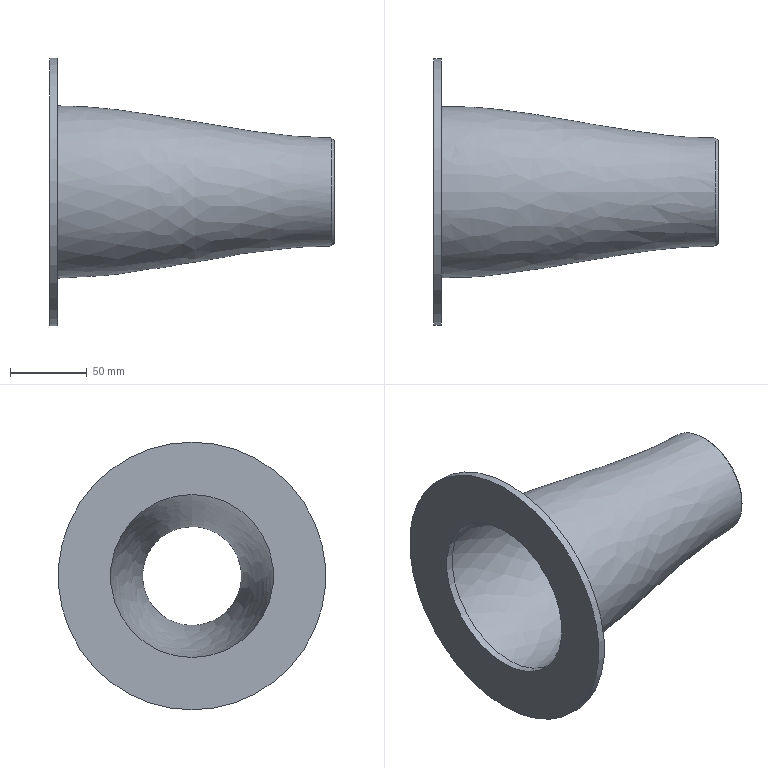Part | STEP file | Reducer Primary Air | 1 solid | 8 faces | box 185 x 174 x 174 mm | volume 225205 mm3 | spline 3 | plane 3 | cylinder 2 | commonest cylinder face diameters 106 x1 174 x1
STEP:
#1=CARTESIAN_POINT('',(-39.149,-5.906,13.134));
#2=VERTEX_POINT('',#1);
#3=CARTESIAN_POINT('',(-39.208,-5.906,13.193));
#4=VERTEX_POINT('',#3);
#5=CARTESIAN_POINT('',(-39.149,-5.906,13.134));
#6=DIRECTION('',(-0.7061,0.,0.7081));
#7=VECTOR('',#6,0.3937);
#8=LINE('',#5,#7);
#9=EDGE_CURVE('',#2,#4,#8,.T.);
#10=ORIENTED_EDGE('',*,*,#9,.T.);
#11=CARTESIAN_POINT('',(-39.208,-5.906,13.193));
#12=CARTESIAN_POINT('',(-39.208,-6.112,13.193));
#13=CARTESIAN_POINT('',(-39.208,-6.526,13.099));
#14=CARTESIAN_POINT('',(-39.208,-7.023,12.702));
#15=CARTESIAN_POINT('',(-39.208,-7.299,12.129));
#16=CARTESIAN_POINT('',(-39.208,-7.299,11.564));
#17=CARTESIAN_POINT('',(-39.208,-7.12,11.11));
#18=CARTESIAN_POINT('',(-39.208,-6.86,10.783));
#19=CARTESIAN_POINT('',(-39.208,-6.572,10.586));
#20=CARTESIAN_POINT('',(-39.208,-6.314,10.485));
#21=CARTESIAN_POINT('',(-39.208,-6.045,10.424));
#22=CARTESIAN_POINT('',(-39.208,-5.696,10.424));
#23=CARTESIAN_POINT('',(-39.208,-5.297,10.547));
#24=CARTESIAN_POINT('',(-39.208,-4.951,10.783));
#25=CARTESIAN_POINT('',(-39.208,-4.69,11.11));
#26=CARTESIAN_POINT('',(-39.208,-4.538,11.499));
#27=CARTESIAN_POINT('',(-39.208,-4.495,12.055));
#28=CARTESIAN_POINT('',(-39.208,-4.732,12.658));
#29=CARTESIAN_POINT('',(-39.208,-5.286,13.099));
#30=CARTESIAN_POINT('',(-39.208,-5.699,13.193));
#31=CARTESIAN_POINT('',(-39.208,-5.906,13.193));
#32=B_SPLINE_CURVE_WITH_KNOTS('',3,(#11,#12,#13,#14,#15,#16,#17,#18,#19,#20,#21,#22,#23,#24,#25,#26,#27,#28,#29,#30,#31),.UNSPECIFIED.,.T.,.F.,(4,1,1,1,1,1,1,1,1,1,1,1,1,1,1,1,1,1,4),(-3.142,-2.693,-2.244,-1.795,-1.346,-1.047,-0.748,-0.4488,-0.2992,-0.1496,0.1496,0.4488,0.748,1.047,1.346,1.646,2.244,2.693,3.142),.UNSPECIFIED.);
#33=EDGE_CURVE('',#4,#4,#32,.T.);
#34=ORIENTED_EDGE('',*,*,#33,.T.);
#35=ORIENTED_EDGE('',*,*,#9,.F.);
#36=CARTESIAN_POINT('',(-39.149,-5.906,13.134));
#37=CARTESIAN_POINT('',(-39.149,-5.708,13.134));
#38=CARTESIAN_POINT('',(-39.149,-5.312,13.043));
#39=CARTESIAN_POINT('',(-39.149,-4.782,12.622));
#40=CARTESIAN_POINT('',(-39.149,-4.556,12.045));
#41=CARTESIAN_POINT('',(-39.149,-4.597,11.512));
#42=CARTESIAN_POINT('',(-39.149,-4.743,11.14));
#43=CARTESIAN_POINT('',(-39.149,-4.992,10.827));
#44=CARTESIAN_POINT('',(-39.149,-5.323,10.601));
#45=CARTESIAN_POINT('',(-39.149,-5.705,10.483));
#46=CARTESIAN_POINT('',(-39.149,-6.039,10.483));
#47=CARTESIAN_POINT('',(-39.149,-6.297,10.542));
#48=CARTESIAN_POINT('',(-39.149,-6.543,10.639));
#49=CARTESIAN_POINT('',(-39.149,-6.819,10.827));
#50=CARTESIAN_POINT('',(-39.149,-7.068,11.14));
#51=CARTESIAN_POINT('',(-39.149,-7.239,11.574));
#52=CARTESIAN_POINT('',(-39.149,-7.239,12.115));
#53=CARTESIAN_POINT('',(-39.149,-6.975,12.664));
#54=CARTESIAN_POINT('',(-39.149,-6.499,13.044));
#55=CARTESIAN_POINT('',(-39.149,-6.103,13.134));
#56=CARTESIAN_POINT('',(-39.149,-5.906,13.134));
#57=B_SPLINE_CURVE_WITH_KNOTS('',3,(#36,#37,#38,#39,#40,#41,#42,#43,#44,#45,#46,#47,#48,#49,#50,#51,#52,#53,#54,#55,#56),.UNSPECIFIED.,.T.,.F.,(4,1,1,1,1,1,1,1,1,1,1,1,1,1,1,1,1,1,4),(-3.142,-2.693,-2.244,-1.646,-1.346,-1.047,-0.748,-0.4488,-0.1496,0.1496,0.2992,0.4488,0.748,1.047,1.346,1.795,2.244,2.693,3.142),.UNSPECIFIED.);
#58=EDGE_CURVE('',#2,#2,#57,.T.);
#59=ORIENTED_EDGE('',*,*,#58,.T.);
#60=EDGE_LOOP('',(#10,#34,#35,#59));
#61=FACE_OUTER_BOUND('',#60,.T.);
#62=CARTESIAN_POINT('',(-39.149,-5.906,13.134));
#63=CARTESIAN_POINT('',(-39.149,-6.103,13.134));
#64=CARTESIAN_POINT('',(-39.149,-6.499,13.044));
#65=CARTESIAN_POINT('',(-39.149,-6.975,12.664));
#66=CARTESIAN_POINT('',(-39.149,-7.239,12.115));
#67=CARTESIAN_POINT('',(-39.149,-7.239,11.574));
#68=CARTESIAN_POINT('',(-39.149,-7.068,11.14));
#69=CARTESIAN_POINT('',(-39.149,-6.819,10.827));
#70=CARTESIAN_POINT('',(-39.149,-6.543,10.639));
#71=CARTESIAN_POINT('',(-39.149,-6.297,10.542));
#72=CARTESIAN_POINT('',(-39.149,-6.039,10.483));
#73=CARTESIAN_POINT('',(-39.149,-5.705,10.483));
#74=CARTESIAN_POINT('',(-39.149,-5.323,10.601));
#75=CARTESIAN_POINT('',(-39.149,-4.992,10.827));
#76=CARTESIAN_POINT('',(-39.149,-4.743,11.14));
#77=CARTESIAN_POINT('',(-39.149,-4.597,11.512));
#78=CARTESIAN_POINT('',(-39.149,-4.556,12.045));
#79=CARTESIAN_POINT('',(-39.149,-4.782,12.622));
#80=CARTESIAN_POINT('',(-39.149,-5.312,13.043));
#81=CARTESIAN_POINT('',(-39.149,-5.708,13.134));
#82=CARTESIAN_POINT('',(-39.149,-5.906,13.134));
#83=CARTESIAN_POINT('',(-39.169,-5.906,13.154));
#84=CARTESIAN_POINT('',(-39.169,-6.106,13.154));
#85=CARTESIAN_POINT('',(-39.169,-6.508,13.062));
#86=CARTESIAN_POINT('',(-39.169,-6.991,12.677));
#87=CARTESIAN_POINT('',(-39.169,-7.259,12.12));
#88=CARTESIAN_POINT('',(-39.169,-7.259,11.571));
#89=CARTESIAN_POINT('',(-39.169,-7.086,11.13));
#90=CARTESIAN_POINT('',(-39.169,-6.832,10.812));
#91=CARTESIAN_POINT('',(-39.169,-6.553,10.621));
#92=CARTESIAN_POINT('',(-39.169,-6.303,10.523));
#93=CARTESIAN_POINT('',(-39.169,-6.041,10.463));
#94=CARTESIAN_POINT('',(-39.169,-5.702,10.463));
#95=CARTESIAN_POINT('',(-39.169,-5.314,10.583));
#96=CARTESIAN_POINT('',(-39.169,-4.979,10.812));
#97=CARTESIAN_POINT('',(-39.169,-4.725,11.13));
#98=CARTESIAN_POINT('',(-39.169,-4.577,11.508));
#99=CARTESIAN_POINT('',(-39.169,-4.536,12.048));
#100=CARTESIAN_POINT('',(-39.169,-4.765,12.634));
#101=CARTESIAN_POINT('',(-39.169,-5.304,13.062));
#102=CARTESIAN_POINT('',(-39.169,-5.705,13.154));
#103=CARTESIAN_POINT('',(-39.169,-5.906,13.154));
#104=CARTESIAN_POINT('',(-39.189,-5.906,13.173));
#105=CARTESIAN_POINT('',(-39.189,-6.109,13.173));
#106=CARTESIAN_POINT('',(-39.189,-6.517,13.08));
#107=CARTESIAN_POINT('',(-39.189,-7.007,12.689));
#108=CARTESIAN_POINT('',(-39.189,-7.279,12.124));
#109=CARTESIAN_POINT('',(-39.189,-7.279,11.567));
#110=CARTESIAN_POINT('',(-39.189,-7.103,11.12));
#111=CARTESIAN_POINT('',(-39.189,-6.846,10.797));
#112=CARTESIAN_POINT('',(-39.189,-6.562,10.604));
#113=CARTESIAN_POINT('',(-39.189,-6.309,10.504));
#114=CARTESIAN_POINT('',(-39.189,-6.043,10.444));
#115=CARTESIAN_POINT('',(-39.189,-5.699,10.444));
#116=CARTESIAN_POINT('',(-39.189,-5.305,10.565));
#117=CARTESIAN_POINT('',(-39.189,-4.965,10.797));
#118=CARTESIAN_POINT('',(-39.189,-4.708,11.12));
#119=CARTESIAN_POINT('',(-39.189,-4.558,11.503));
#120=CARTESIAN_POINT('',(-39.189,-4.515,12.052));
#121=CARTESIAN_POINT('',(-39.189,-4.749,12.646));
#122=CARTESIAN_POINT('',(-39.189,-5.295,13.08));
#123=CARTESIAN_POINT('',(-39.189,-5.702,13.173));
#124=CARTESIAN_POINT('',(-39.189,-5.906,13.173));
#125=CARTESIAN_POINT('',(-39.208,-5.906,13.193));
#126=CARTESIAN_POINT('',(-39.208,-6.112,13.193));
#127=CARTESIAN_POINT('',(-39.208,-6.526,13.099));
#128=CARTESIAN_POINT('',(-39.208,-7.023,12.702));
#129=CARTESIAN_POINT('',(-39.208,-7.299,12.129));
#130=CARTESIAN_POINT('',(-39.208,-7.299,11.564));
#131=CARTESIAN_POINT('',(-39.208,-7.12,11.11));
#132=CARTESIAN_POINT('',(-39.208,-6.86,10.783));
#133=CARTESIAN_POINT('',(-39.208,-6.572,10.586));
#134=CARTESIAN_POINT('',(-39.208,-6.314,10.485));
#135=CARTESIAN_POINT('',(-39.208,-6.045,10.424));
#136=CARTESIAN_POINT('',(-39.208,-5.696,10.424));
#137=CARTESIAN_POINT('',(-39.208,-5.297,10.547));
#138=CARTESIAN_POINT('',(-39.208,-4.951,10.783));
#139=CARTESIAN_POINT('',(-39.208,-4.69,11.11));
#140=CARTESIAN_POINT('',(-39.208,-4.538,11.499));
#141=CARTESIAN_POINT('',(-39.208,-4.495,12.055));
#142=CARTESIAN_POINT('',(-39.208,-4.732,12.658));
#143=CARTESIAN_POINT('',(-39.208,-5.286,13.099));
#144=CARTESIAN_POINT('',(-39.208,-5.699,13.193));
#145=CARTESIAN_POINT('',(-39.208,-5.906,13.193));
#146=B_SPLINE_SURFACE_WITH_KNOTS('',3,3,((#62,#63,#64,#65,#66,#67,#68,#69,#70,#71,#72,#73,#74,#75,#76,#77,#78,#79,#80,#81,#82),(#83,#84,#85,#86,#87,#88,#89,#90,#91,#92,#93,#94,#95,#96,#97,#98,#99,#100,#101,#102,#103),(#104,#105,#106,#107,#108,#109,#110,#111,#112,#113,#114,#115,#116,#117,#118,#119,#120,#121,#122,#123,#124),(#125,#126,#127,#128,#129,#130,#131,#132,#133,#134,#135,#136,#137,#138,#139,#140,#141,#142,#143,#144,#145)),.UNSPECIFIED.,.F.,.T.,.F.,(4,4),(4,1,1,1,1,1,1,1,1,1,1,1,1,1,1,1,1,1,4),(0.,1.),(-3.142,-2.693,-2.244,-1.795,-1.346,-1.047,-0.748,-0.4488,-0.2992,-0.1496,0.1496,0.4488,0.748,1.047,1.346,1.646,2.244,2.693,3.142),.UNSPECIFIED.);
#147=ADVANCED_FACE('',(#61),#146,.T.);
#148=ORIENTED_EDGE('',*,*,#33,.F.);
#149=CARTESIAN_POINT('',(-46.236,-5.906,14.016));
#150=VERTEX_POINT('',#149);
#151=CARTESIAN_POINT('',(-39.208,-5.906,13.193));
#152=CARTESIAN_POINT('',(-41.551,-5.906,13.207));
#153=CARTESIAN_POINT('',(-43.893,-5.906,14.016));
#154=CARTESIAN_POINT('',(-46.236,-5.906,14.016));
#155=B_SPLINE_CURVE_WITH_KNOTS('',3,(#151,#152,#153,#154),.UNSPECIFIED.,.F.,.F.,(4,4),(0.008333,1.),.UNSPECIFIED.);
#156=EDGE_CURVE('',#4,#150,#155,.T.);
#157=ORIENTED_EDGE('',*,*,#156,.T.);
#158=CARTESIAN_POINT('',(-46.236,-5.906,11.811));
#159=DIRECTION('',(1.,0.,0.));
#160=DIRECTION('',(0.,0.,-1.));
#161=AXIS2_PLACEMENT_3D('',#158,#159,#160);
#162=CIRCLE('',#161,2.205);
#163=EDGE_CURVE('',#150,#150,#162,.T.);
#164=ORIENTED_EDGE('',*,*,#163,.T.);
#165=ORIENTED_EDGE('',*,*,#156,.F.);
#166=EDGE_LOOP('',(#148,#157,#164,#165));
#167=FACE_OUTER_BOUND('',#166,.T.);
#168=CARTESIAN_POINT('',(-39.208,-5.906,13.193));
#169=CARTESIAN_POINT('',(-41.551,-5.906,13.207));
#170=CARTESIAN_POINT('',(-43.893,-5.906,14.016));
#171=CARTESIAN_POINT('',(-46.236,-5.906,14.016));
#172=CARTESIAN_POINT('',(-39.208,-6.112,13.193));
#173=CARTESIAN_POINT('',(-41.551,-6.114,13.207));
#174=CARTESIAN_POINT('',(-43.893,-6.235,14.016));
#175=CARTESIAN_POINT('',(-46.236,-6.235,14.016));
#176=CARTESIAN_POINT('',(-39.208,-6.526,13.099));
#177=CARTESIAN_POINT('',(-41.551,-6.532,13.111));
#178=CARTESIAN_POINT('',(-43.893,-6.895,13.865));
#179=CARTESIAN_POINT('',(-46.236,-6.895,13.865));
#180=CARTESIAN_POINT('',(-39.208,-6.968,12.746));
#181=CARTESIAN_POINT('',(-41.551,-6.978,12.755));
#182=CARTESIAN_POINT('',(-43.893,-7.6,13.303));
#183=CARTESIAN_POINT('',(-46.236,-7.6,13.303));
#184=CARTESIAN_POINT('',(-39.208,-7.211,12.323));
#185=CARTESIAN_POINT('',(-41.551,-7.224,12.328));
#186=CARTESIAN_POINT('',(-43.893,-7.989,12.628));
#187=CARTESIAN_POINT('',(-46.236,-7.989,12.628));
#188=CARTESIAN_POINT('',(-39.208,-7.304,11.916));
#189=CARTESIAN_POINT('',(-41.551,-7.318,11.917));
#190=CARTESIAN_POINT('',(-43.893,-8.137,11.978));
#191=CARTESIAN_POINT('',(-46.236,-8.137,11.978));
#192=CARTESIAN_POINT('',(-39.208,-7.273,11.499));
#193=CARTESIAN_POINT('',(-41.551,-7.286,11.496));
#194=CARTESIAN_POINT('',(-43.893,-8.087,11.313));
#195=CARTESIAN_POINT('',(-46.236,-8.087,11.313));
#196=CARTESIAN_POINT('',(-39.208,-7.12,11.11));
#197=CARTESIAN_POINT('',(-41.551,-7.132,11.103));
#198=CARTESIAN_POINT('',(-43.893,-7.844,10.692));
#199=CARTESIAN_POINT('',(-46.236,-7.844,10.692));
#200=CARTESIAN_POINT('',(-39.208,-6.86,10.783));
#201=CARTESIAN_POINT('',(-41.551,-6.869,10.773));
#202=CARTESIAN_POINT('',(-43.893,-7.428,10.171));
#203=CARTESIAN_POINT('',(-46.236,-7.428,10.171));
#204=CARTESIAN_POINT('',(-39.208,-6.514,10.547));
#205=CARTESIAN_POINT('',(-41.551,-6.52,10.535));
#206=CARTESIAN_POINT('',(-43.893,-6.876,9.795));
#207=CARTESIAN_POINT('',(-46.236,-6.876,9.795));
#208=CARTESIAN_POINT('',(-39.208,-6.115,10.424));
#209=CARTESIAN_POINT('',(-41.551,-6.117,10.41));
#210=CARTESIAN_POINT('',(-43.893,-6.239,9.598));
#211=CARTESIAN_POINT('',(-46.236,-6.239,9.598));
#212=CARTESIAN_POINT('',(-39.208,-5.696,10.424));
#213=CARTESIAN_POINT('',(-41.551,-5.694,10.41));
#214=CARTESIAN_POINT('',(-43.893,-5.572,9.598));
#215=CARTESIAN_POINT('',(-46.236,-5.572,9.598));
#216=CARTESIAN_POINT('',(-39.208,-5.297,10.547));
#217=CARTESIAN_POINT('',(-41.551,-5.291,10.535));
#218=CARTESIAN_POINT('',(-43.893,-4.934,9.795));
#219=CARTESIAN_POINT('',(-46.236,-4.934,9.795));
#220=CARTESIAN_POINT('',(-39.208,-4.951,10.783));
#221=CARTESIAN_POINT('',(-41.551,-4.942,10.773));
#222=CARTESIAN_POINT('',(-43.893,-4.383,10.17));
#223=CARTESIAN_POINT('',(-46.236,-4.383,10.17));
#224=CARTESIAN_POINT('',(-39.208,-4.691,11.11));
#225=CARTESIAN_POINT('',(-41.551,-4.679,11.103));
#226=CARTESIAN_POINT('',(-43.893,-3.967,10.692));
#227=CARTESIAN_POINT('',(-46.236,-3.967,10.692));
#228=CARTESIAN_POINT('',(-39.208,-4.512,11.564));
#229=CARTESIAN_POINT('',(-41.551,-4.499,11.561));
#230=CARTESIAN_POINT('',(-43.893,-3.683,11.416));
#231=CARTESIAN_POINT('',(-46.236,-3.683,11.416));
#232=CARTESIAN_POINT('',(-39.208,-4.512,12.129));
#233=CARTESIAN_POINT('',(-41.551,-4.498,12.132));
#234=CARTESIAN_POINT('',(-43.893,-3.683,12.318));
#235=CARTESIAN_POINT('',(-46.236,-3.683,12.318));
#236=CARTESIAN_POINT('',(-39.208,-4.788,12.702));
#237=CARTESIAN_POINT('',(-41.551,-4.777,12.711));
#238=CARTESIAN_POINT('',(-43.893,-4.123,13.233));
#239=CARTESIAN_POINT('',(-46.236,-4.123,13.233));
#240=CARTESIAN_POINT('',(-39.208,-5.285,13.099));
#241=CARTESIAN_POINT('',(-41.551,-5.279,13.111));
#242=CARTESIAN_POINT('',(-43.893,-4.916,13.865));
#243=CARTESIAN_POINT('',(-46.236,-4.916,13.865));
#244=CARTESIAN_POINT('',(-39.208,-5.699,13.193));
#245=CARTESIAN_POINT('',(-41.551,-5.697,13.207));
#246=CARTESIAN_POINT('',(-43.893,-5.576,14.016));
#247=CARTESIAN_POINT('',(-46.236,-5.576,14.016));
#248=CARTESIAN_POINT('',(-39.208,-5.906,13.193));
#249=CARTESIAN_POINT('',(-41.551,-5.906,13.207));
#250=CARTESIAN_POINT('',(-43.893,-5.906,14.016));
#251=CARTESIAN_POINT('',(-46.236,-5.906,14.016));
#252=B_SPLINE_SURFACE_WITH_KNOTS('',3,3,((#168,#169,#170,#171),(#172,#173,#174,#175),(#176,#177,#178,#179),(#180,#181,#182,#183),(#184,#185,#186,#187),(#188,#189,#190,#191),(#192,#193,#194,#195),(#196,#197,#198,#199),(#200,#201,#202,#203),(#204,#205,#206,#207),(#208,#209,#210,#211),(#212,#213,#214,#215),(#216,#217,#218,#219),(#220,#221,#222,#223),(#224,#225,#226,#227),(#228,#229,#230,#231),(#232,#233,#234,#235),(#236,#237,#238,#239),(#240,#241,#242,#243),(#244,#245,#246,#247),(#248,#249,#250,#251)),.UNSPECIFIED.,.T.,.F.,.F.,(4,1,1,1,1,1,1,1,1,1,1,1,1,1,1,1,1,1,4),(4,4),(0.,0.07143,0.1429,0.1905,0.2381,0.2857,0.3333,0.381,0.4286,0.4762,0.5238,0.5714,0.619,0.6667,0.7143,0.7857,0.8571,0.9286,1.),(0.008333,1.),.UNSPECIFIED.);
#253=ADVANCED_FACE('',(#167),#252,.F.);
#254=ORIENTED_EDGE('',*,*,#58,.F.);
#255=EDGE_LOOP('',(#254));
#256=FACE_OUTER_BOUND('',#255,.T.);
#257=CARTESIAN_POINT('',(-39.149,-5.906,13.075));
#258=VERTEX_POINT('',#257);
#259=CARTESIAN_POINT('',(-39.149,-5.906,13.075));
#260=CARTESIAN_POINT('',(-39.149,-5.716,13.075));
#261=CARTESIAN_POINT('',(-39.149,-5.338,12.989));
#262=CARTESIAN_POINT('',(-39.149,-4.884,12.626));
#263=CARTESIAN_POINT('',(-39.149,-4.631,12.102));
#264=CARTESIAN_POINT('',(-39.149,-4.631,11.585));
#265=CARTESIAN_POINT('',(-39.149,-4.795,11.17));
#266=CARTESIAN_POINT('',(-39.149,-5.033,10.871));
#267=CARTESIAN_POINT('',(-39.149,-5.349,10.655));
#268=CARTESIAN_POINT('',(-39.149,-5.714,10.543));
#269=CARTESIAN_POINT('',(-39.149,-6.097,10.543));
#270=CARTESIAN_POINT('',(-39.149,-6.462,10.655));
#271=CARTESIAN_POINT('',(-39.149,-6.778,10.871));
#272=CARTESIAN_POINT('',(-39.149,-7.016,11.17));
#273=CARTESIAN_POINT('',(-39.149,-7.156,11.526));
#274=CARTESIAN_POINT('',(-39.149,-7.185,11.907));
#275=CARTESIAN_POINT('',(-39.149,-7.1,12.28));
#276=CARTESIAN_POINT('',(-39.149,-6.877,12.666));
#277=CARTESIAN_POINT('',(-39.149,-6.473,12.989));
#278=CARTESIAN_POINT('',(-39.149,-6.095,13.075));
#279=CARTESIAN_POINT('',(-39.149,-5.906,13.075));
#280=B_SPLINE_CURVE_WITH_KNOTS('',3,(#259,#260,#261,#262,#263,#264,#265,#266,#267,#268,#269,#270,#271,#272,#273,#274,#275,#276,#277,#278,#279),.UNSPECIFIED.,.T.,.F.,(4,1,1,1,1,1,1,1,1,1,1,1,1,1,1,1,1,1,4),(-1.,-0.9286,-0.8571,-0.7857,-0.7143,-0.6667,-0.619,-0.5714,-0.5238,-0.4762,-0.4286,-0.381,-0.3333,-0.2857,-0.2381,-0.1905,-0.1429,-0.07143,0.),.UNSPECIFIED.);
#281=EDGE_CURVE('',#258,#258,#280,.T.);
#282=ORIENTED_EDGE('',*,*,#281,.T.);
#283=EDGE_LOOP('',(#282));
#284=FACE_BOUND('',#283,.T.);
#285=CARTESIAN_POINT('',(-39.149,-5.906,11.811));
#286=DIRECTION('',(1.,0.,0.));
#287=DIRECTION('',(0.,0.,-1.));
#288=AXIS2_PLACEMENT_3D('',#285,#286,#287);
#289=PLANE('',#288);
#290=ADVANCED_FACE('',(#256,#284),#289,.T.);
#291=CARTESIAN_POINT('',(-46.236,-5.906,8.386));
#292=VERTEX_POINT('',#291);
#293=CARTESIAN_POINT('',(-46.236,-5.906,11.811));
#294=DIRECTION('',(1.,0.,0.));
#295=DIRECTION('',(0.,0.,1.));
#296=AXIS2_PLACEMENT_3D('',#293,#294,#295);
#297=CIRCLE('',#296,3.425);
#298=EDGE_CURVE('',#292,#292,#297,.T.);
#299=ORIENTED_EDGE('',*,*,#298,.F.);
#300=CARTESIAN_POINT('',(-46.433,-5.906,8.386));
#301=VERTEX_POINT('',#300);
#302=CARTESIAN_POINT('',(-46.433,-5.906,8.386));
#303=DIRECTION('',(-1.,0.,0.));
#304=VECTOR('',#303,3.425);
#305=LINE('',#302,#304);
#306=EDGE_CURVE('',#292,#301,#305,.T.);
#307=ORIENTED_EDGE('',*,*,#306,.T.);
#308=CARTESIAN_POINT('',(-46.433,-5.906,11.811));
#309=DIRECTION('',(-1.,0.,0.));
#310=DIRECTION('',(0.,0.,1.));
#311=AXIS2_PLACEMENT_3D('',#308,#309,#310);
#312=CIRCLE('',#311,3.425);
#313=EDGE_CURVE('',#301,#301,#312,.T.);
#314=ORIENTED_EDGE('',*,*,#313,.F.);
#315=ORIENTED_EDGE('',*,*,#306,.F.);
#316=EDGE_LOOP('',(#299,#307,#314,#315));
#317=FACE_OUTER_BOUND('',#316,.T.);
#318=CARTESIAN_POINT('',(-46.433,-5.906,11.811));
#319=DIRECTION('',(1.,0.,0.));
#320=DIRECTION('',(0.,0.,1.));
#321=AXIS2_PLACEMENT_3D('',#318,#319,#320);
#322=CYLINDRICAL_SURFACE('',#321,3.425);
#323=ADVANCED_FACE('',(#317),#322,.T.);
#324=ORIENTED_EDGE('',*,*,#298,.T.);
#325=EDGE_LOOP('',(#324));
#326=FACE_OUTER_BOUND('',#325,.T.);
#327=ORIENTED_EDGE('',*,*,#163,.F.);
#328=EDGE_LOOP('',(#327));
#329=FACE_BOUND('',#328,.T.);
#330=CARTESIAN_POINT('',(-46.236,-5.906,11.811));
#331=DIRECTION('',(-1.,0.,0.));
#332=DIRECTION('',(0.,0.,1.));
#333=AXIS2_PLACEMENT_3D('',#330,#331,#332);
#334=PLANE('',#333);
#335=ADVANCED_FACE('',(#326,#329),#334,.F.);
#336=CARTESIAN_POINT('',(-46.236,-5.906,13.898));
#337=VERTEX_POINT('',#336);
#338=CARTESIAN_POINT('',(-46.236,-5.906,9.724));
#339=VERTEX_POINT('',#338);
#340=CARTESIAN_POINT('',(-46.236,-5.906,11.811));
#341=DIRECTION('',(1.,0.,0.));
#342=DIRECTION('',(0.,0.,-1.));
#343=AXIS2_PLACEMENT_3D('',#340,#341,#342);
#344=CIRCLE('',#343,2.087);
#345=EDGE_CURVE('',#337,#339,#344,.T.);
#346=ORIENTED_EDGE('',*,*,#345,.T.);
#347=CARTESIAN_POINT('',(-46.433,-5.906,9.724));
#348=VERTEX_POINT('',#347);
#349=CARTESIAN_POINT('',(-46.236,-5.906,9.724));
#350=DIRECTION('',(-1.,0.,0.));
#351=VECTOR('',#350,2.205);
#352=LINE('',#349,#351);
#353=EDGE_CURVE('',#339,#348,#352,.T.);
#354=ORIENTED_EDGE('',*,*,#353,.T.);
#355=CARTESIAN_POINT('',(-46.433,-5.906,11.811));
#356=DIRECTION('',(1.,0.,0.));
#357=DIRECTION('',(0.,0.,1.));
#358=AXIS2_PLACEMENT_3D('',#355,#356,#357);
#359=CIRCLE('',#358,2.087);
#360=EDGE_CURVE('',#348,#348,#359,.T.);
#361=ORIENTED_EDGE('',*,*,#360,.F.);
#362=ORIENTED_EDGE('',*,*,#353,.F.);
#363=CARTESIAN_POINT('',(-46.236,-5.906,11.811));
#364=DIRECTION('',(1.,0.,0.));
#365=DIRECTION('',(0.,0.,-1.));
#366=AXIS2_PLACEMENT_3D('',#363,#364,#365);
#367=CIRCLE('',#366,2.087);
#368=EDGE_CURVE('',#339,#337,#367,.T.);
#369=ORIENTED_EDGE('',*,*,#368,.T.);
#370=EDGE_LOOP('',(#346,#354,#361,#362,#369));
#371=FACE_OUTER_BOUND('',#370,.T.);
#372=CARTESIAN_POINT('',(-46.236,-5.906,11.811));
#373=DIRECTION('',(-1.,0.,0.));
#374=DIRECTION('',(0.,0.,1.));
#375=AXIS2_PLACEMENT_3D('',#372,#373,#374);
#376=CYLINDRICAL_SURFACE('',#375,2.087);
#377=ADVANCED_FACE('',(#371),#376,.F.);
#378=ORIENTED_EDGE('',*,*,#281,.F.);
#379=CARTESIAN_POINT('',(-39.149,-5.906,13.075));
#380=CARTESIAN_POINT('',(-40.515,-5.906,13.075));
#381=CARTESIAN_POINT('',(-42.888,-5.906,13.548));
#382=CARTESIAN_POINT('',(-45.235,-5.906,13.898));
#383=CARTESIAN_POINT('',(-46.236,-5.906,13.898));
#384=B_SPLINE_CURVE_WITH_KNOTS('',3,(#379,#380,#381,#382,#383),.UNSPECIFIED.,.F.,.F.,(4,1,4),(0.,0.5714,1.),.UNSPECIFIED.);
#385=EDGE_CURVE('',#258,#337,#384,.T.);
#386=ORIENTED_EDGE('',*,*,#385,.T.);
#387=ORIENTED_EDGE('',*,*,#368,.F.);
#388=ORIENTED_EDGE('',*,*,#345,.F.);
#389=ORIENTED_EDGE('',*,*,#385,.F.);
#390=EDGE_LOOP('',(#378,#386,#387,#388,#389));
#391=FACE_OUTER_BOUND('',#390,.T.);
#392=CARTESIAN_POINT('',(-39.149,-5.906,13.075));
#393=CARTESIAN_POINT('',(-40.515,-5.906,13.075));
#394=CARTESIAN_POINT('',(-42.888,-5.906,13.548));
#395=CARTESIAN_POINT('',(-45.235,-5.906,13.898));
#396=CARTESIAN_POINT('',(-46.236,-5.906,13.898));
#397=CARTESIAN_POINT('',(-39.149,-6.095,13.075));
#398=CARTESIAN_POINT('',(-40.515,-6.095,13.075));
#399=CARTESIAN_POINT('',(-42.888,-6.165,13.548));
#400=CARTESIAN_POINT('',(-45.235,-6.218,13.898));
#401=CARTESIAN_POINT('',(-46.236,-6.218,13.898));
#402=CARTESIAN_POINT('',(-39.149,-6.473,12.989));
#403=CARTESIAN_POINT('',(-40.515,-6.473,12.989));
#404=CARTESIAN_POINT('',(-42.888,-6.685,13.43));
#405=CARTESIAN_POINT('',(-45.235,-6.842,13.755));
#406=CARTESIAN_POINT('',(-46.236,-6.842,13.755));
#407=CARTESIAN_POINT('',(-39.149,-6.877,12.666));
#408=CARTESIAN_POINT('',(-40.515,-6.877,12.666));
#409=CARTESIAN_POINT('',(-42.888,-7.241,12.987));
#410=CARTESIAN_POINT('',(-45.235,-7.509,13.223));
#411=CARTESIAN_POINT('',(-46.236,-7.509,13.223));
#412=CARTESIAN_POINT('',(-39.149,-7.1,12.28));
#413=CARTESIAN_POINT('',(-40.515,-7.1,12.28));
#414=CARTESIAN_POINT('',(-42.888,-7.547,12.455));
#415=CARTESIAN_POINT('',(-45.235,-7.877,12.585));
#416=CARTESIAN_POINT('',(-46.236,-7.877,12.585));
#417=CARTESIAN_POINT('',(-39.149,-7.185,11.907));
#418=CARTESIAN_POINT('',(-40.515,-7.185,11.907));
#419=CARTESIAN_POINT('',(-42.888,-7.664,11.943));
#420=CARTESIAN_POINT('',(-45.235,-8.018,11.969));
#421=CARTESIAN_POINT('',(-46.236,-8.018,11.969));
#422=CARTESIAN_POINT('',(-39.149,-7.156,11.526));
#423=CARTESIAN_POINT('',(-40.515,-7.156,11.526));
#424=CARTESIAN_POINT('',(-42.888,-7.625,11.419));
#425=CARTESIAN_POINT('',(-45.235,-7.97,11.34));
#426=CARTESIAN_POINT('',(-46.236,-7.97,11.34));
#427=CARTESIAN_POINT('',(-39.149,-7.016,11.17));
#428=CARTESIAN_POINT('',(-40.515,-7.016,11.17));
#429=CARTESIAN_POINT('',(-42.888,-7.433,10.929));
#430=CARTESIAN_POINT('',(-45.235,-7.74,10.752));
#431=CARTESIAN_POINT('',(-46.236,-7.74,10.752));
#432=CARTESIAN_POINT('',(-39.149,-6.778,10.871));
#433=CARTESIAN_POINT('',(-40.515,-6.778,10.871));
#434=CARTESIAN_POINT('',(-42.888,-7.105,10.518));
#435=CARTESIAN_POINT('',(-45.235,-7.346,10.258));
#436=CARTESIAN_POINT('',(-46.236,-7.346,10.258));
#437=CARTESIAN_POINT('',(-39.149,-6.462,10.655));
#438=CARTESIAN_POINT('',(-40.515,-6.462,10.655));
#439=CARTESIAN_POINT('',(-42.888,-6.671,10.222));
#440=CARTESIAN_POINT('',(-45.235,-6.824,9.903));
#441=CARTESIAN_POINT('',(-46.236,-6.824,9.903));
#442=CARTESIAN_POINT('',(-39.149,-6.097,10.543));
#443=CARTESIAN_POINT('',(-40.515,-6.097,10.543));
#444=CARTESIAN_POINT('',(-42.888,-6.168,10.067));
#445=CARTESIAN_POINT('',(-45.235,-6.221,9.717));
#446=CARTESIAN_POINT('',(-46.236,-6.221,9.717));
#447=CARTESIAN_POINT('',(-39.149,-5.714,10.543));
#448=CARTESIAN_POINT('',(-40.515,-5.714,10.543));
#449=CARTESIAN_POINT('',(-42.888,-5.643,10.067));
#450=CARTESIAN_POINT('',(-45.235,-5.59,9.717));
#451=CARTESIAN_POINT('',(-46.236,-5.59,9.717));
#452=CARTESIAN_POINT('',(-39.149,-5.349,10.655));
#453=CARTESIAN_POINT('',(-40.515,-5.349,10.655));
#454=CARTESIAN_POINT('',(-42.888,-5.14,10.222));
#455=CARTESIAN_POINT('',(-45.235,-4.987,9.903));
#456=CARTESIAN_POINT('',(-46.236,-4.987,9.903));
#457=CARTESIAN_POINT('',(-39.149,-5.033,10.871));
#458=CARTESIAN_POINT('',(-40.515,-5.033,10.871));
#459=CARTESIAN_POINT('',(-42.888,-4.706,10.518));
#460=CARTESIAN_POINT('',(-45.235,-4.465,10.258));
#461=CARTESIAN_POINT('',(-46.236,-4.465,10.258));
#462=CARTESIAN_POINT('',(-39.149,-4.795,11.17));
#463=CARTESIAN_POINT('',(-40.515,-4.795,11.17));
#464=CARTESIAN_POINT('',(-42.888,-4.378,10.929));
#465=CARTESIAN_POINT('',(-45.235,-4.071,10.752));
#466=CARTESIAN_POINT('',(-46.236,-4.071,10.752));
#467=CARTESIAN_POINT('',(-39.149,-4.631,11.585));
#468=CARTESIAN_POINT('',(-40.515,-4.631,11.585));
#469=CARTESIAN_POINT('',(-42.888,-4.154,11.5));
#470=CARTESIAN_POINT('',(-45.235,-3.802,11.438));
#471=CARTESIAN_POINT('',(-46.236,-3.802,11.438));
#472=CARTESIAN_POINT('',(-39.149,-4.631,12.102));
#473=CARTESIAN_POINT('',(-40.515,-4.631,12.102));
#474=CARTESIAN_POINT('',(-42.888,-4.154,12.211));
#475=CARTESIAN_POINT('',(-45.235,-3.802,12.291));
#476=CARTESIAN_POINT('',(-46.236,-3.802,12.291));
#477=CARTESIAN_POINT('',(-39.149,-4.884,12.626));
#478=CARTESIAN_POINT('',(-40.515,-4.884,12.626));
#479=CARTESIAN_POINT('',(-42.888,-4.501,12.931));
#480=CARTESIAN_POINT('',(-45.235,-4.218,13.156));
#481=CARTESIAN_POINT('',(-46.236,-4.218,13.156));
#482=CARTESIAN_POINT('',(-39.149,-5.338,12.989));
#483=CARTESIAN_POINT('',(-40.515,-5.338,12.989));
#484=CARTESIAN_POINT('',(-42.888,-5.126,13.43));
#485=CARTESIAN_POINT('',(-45.235,-4.969,13.755));
#486=CARTESIAN_POINT('',(-46.236,-4.969,13.755));
#487=CARTESIAN_POINT('',(-39.149,-5.716,13.075));
#488=CARTESIAN_POINT('',(-40.515,-5.716,13.075));
#489=CARTESIAN_POINT('',(-42.888,-5.646,13.548));
#490=CARTESIAN_POINT('',(-45.235,-5.593,13.898));
#491=CARTESIAN_POINT('',(-46.236,-5.593,13.898));
#492=CARTESIAN_POINT('',(-39.149,-5.906,13.075));
#493=CARTESIAN_POINT('',(-40.515,-5.906,13.075));
#494=CARTESIAN_POINT('',(-42.888,-5.906,13.548));
#495=CARTESIAN_POINT('',(-45.235,-5.906,13.898));
#496=CARTESIAN_POINT('',(-46.236,-5.906,13.898));
#497=B_SPLINE_SURFACE_WITH_KNOTS('',3,3,((#392,#393,#394,#395,#396),(#397,#398,#399,#400,#401),(#402,#403,#404,#405,#406),(#407,#408,#409,#410,#411),(#412,#413,#414,#415,#416),(#417,#418,#419,#420,#421),(#422,#423,#424,#425,#426),(#427,#428,#429,#430,#431),(#432,#433,#434,#435,#436),(#437,#438,#439,#440,#441),(#442,#443,#444,#445,#446),(#447,#448,#449,#450,#451),(#452,#453,#454,#455,#456),(#457,#458,#459,#460,#461),(#462,#463,#464,#465,#466),(#467,#468,#469,#470,#471),(#472,#473,#474,#475,#476),(#477,#478,#479,#480,#481),(#482,#483,#484,#485,#486),(#487,#488,#489,#490,#491),(#492,#493,#494,#495,#496)),.UNSPECIFIED.,.T.,.F.,.F.,(4,1,1,1,1,1,1,1,1,1,1,1,1,1,1,1,1,1,4),(4,1,4),(0.,0.07143,0.1429,0.1905,0.2381,0.2857,0.3333,0.381,0.4286,0.4762,0.5238,0.5714,0.619,0.6667,0.7143,0.7857,0.8571,0.9286,1.),(0.,0.5714,1.),.UNSPECIFIED.);
#498=ADVANCED_FACE('',(#391),#497,.T.);
#499=ORIENTED_EDGE('',*,*,#313,.T.);
#500=EDGE_LOOP('',(#499));
#501=FACE_OUTER_BOUND('',#500,.T.);
#502=ORIENTED_EDGE('',*,*,#360,.T.);
#503=EDGE_LOOP('',(#502));
#504=FACE_BOUND('',#503,.T.);
#505=CARTESIAN_POINT('',(-46.433,-5.906,11.811));
#506=DIRECTION('',(-1.,0.,0.));
#507=DIRECTION('',(0.,0.,1.));
#508=AXIS2_PLACEMENT_3D('',#505,#506,#507);
#509=PLANE('',#508);
#510=ADVANCED_FACE('',(#501,#504),#509,.T.);
#511=CLOSED_SHELL('',(#147,#253,#290,#323,#335,#377,#498,#510));
#512=MANIFOLD_SOLID_BREP('',#511);
#513=(LENGTH_UNIT()NAMED_UNIT(*)SI_UNIT(.MILLI.,.METRE.));
#514=LENGTH_MEASURE_WITH_UNIT(LENGTH_MEASURE(25.4),#513);
#515=DIMENSIONAL_EXPONENTS(1.,0.,0.,0.,0.,0.,0.);
#516=(CONVERSION_BASED_UNIT('inch',#514)LENGTH_UNIT()NAMED_UNIT(#515));
#517=UNCERTAINTY_MEASURE_WITH_UNIT(LENGTH_MEASURE(0.0003937),#516,'','');
#518=(NAMED_UNIT(*)PLANE_ANGLE_UNIT()SI_UNIT($,.RADIAN.));
#519=(NAMED_UNIT(*)SI_UNIT($,.STERADIAN.)SOLID_ANGLE_UNIT());
#520=(GEOMETRIC_REPRESENTATION_CONTEXT(3)GLOBAL_UNCERTAINTY_ASSIGNED_CONTEXT((#517))GLOBAL_UNIT_ASSIGNED_CONTEXT((#516,#518,#519))REPRESENTATION_CONTEXT('',''));
#521=ADVANCED_BREP_SHAPE_REPRESENTATION('',(#512),#520);